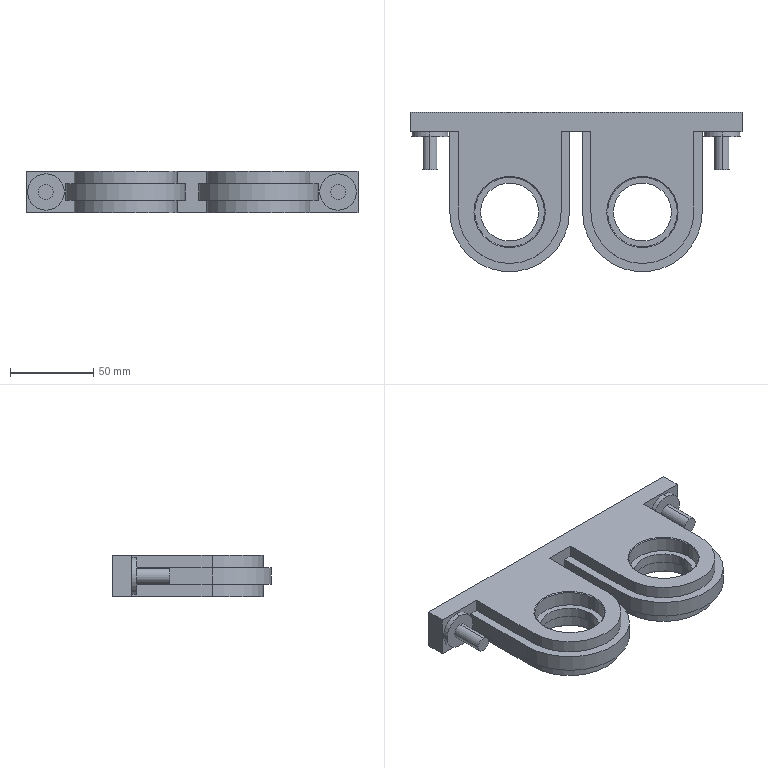Part | SolidWorks | features ICE 2, MoveCopyBody 2, BaseBody 1, CombineBodies 1 | 1 solid | 66 faces | box 200 x 95.96 x 25 mm | volume 244043 mm3 | plane 32 | cylinder 26 | cone 8 | commonest cylinder face diameters 42 x8 9 x4 22 x4 35 x4 62 x4 72 x2